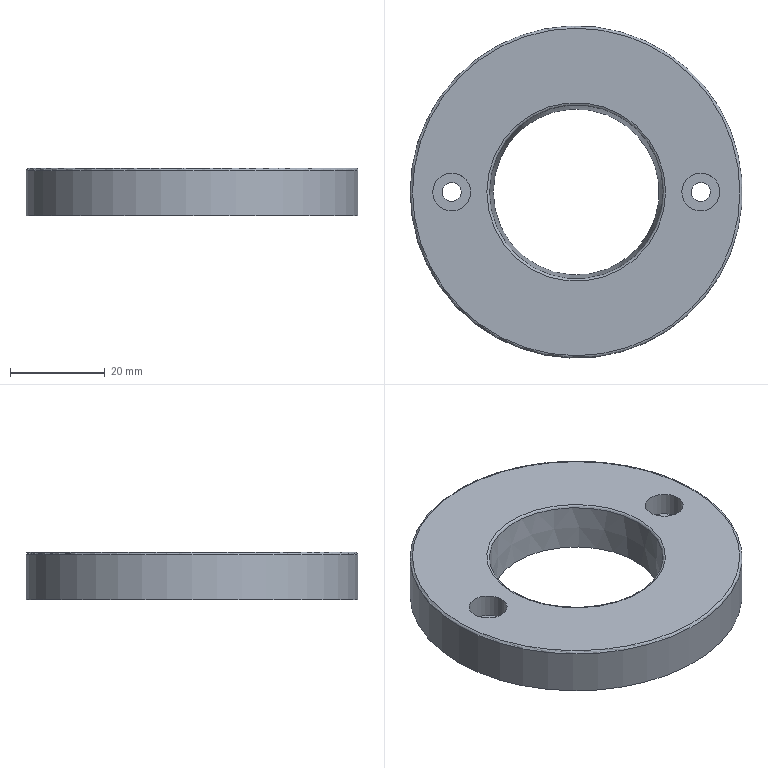Part | STEP file | DISCO_BASE_ALIMENTADOR_ARRUELA | 1 solid | 12 faces | box 70 x 70 x 10 mm | volume 27729 mm3 | cylinder 5 | plane 4 | torus 2 | cone 1 | commonest cylinder face diameters 4 x2 8 x2 70 x1
STEP:
#1=CARTESIAN_POINT('',(0.,0.,0.));
#2=DIRECTION('',(0.,0.,1.));
#3=DIRECTION('',(1.,0.,0.));
#4=AXIS2_PLACEMENT_3D('',#1,#2,#3);
#5=CARTESIAN_POINT('',(-29.76,1.918,5.));
#6=VERTEX_POINT('',#5);
#7=CARTESIAN_POINT('',(-26.25,0.,5.));
#8=DIRECTION('',(0.,0.,-1.));
#9=DIRECTION('',(1.,0.,0.));
#10=AXIS2_PLACEMENT_3D('',#7,#8,#9);
#11=CIRCLE('',#10,4.);
#12=CARTESIAN_POINT('',(-24.25,0.,5.));
#13=DIRECTION('',(0.,0.,-1.));
#14=DIRECTION('',(-1.,0.,0.));
#15=AXIS2_PLACEMENT_3D('',#12,#13,#14);
#16=PLANE('',#15);
#17=CARTESIAN_POINT('',(2.,0.));
#18=DIRECTION('',(-1.,0.));
#19=AXIS2_PLACEMENT_2D('',#17,#18);
#20=CIRCLE('',#19,4.);
#21=(GEOMETRIC_REPRESENTATION_CONTEXT(2)PARAMETRIC_REPRESENTATION_CONTEXT()REPRESENTATION_CONTEXT('',''));
#22=DEFINITIONAL_REPRESENTATION('',(#20),#21);
#23=PCURVE('',#16,#22);
#24=CARTESIAN_POINT('',(-26.25,0.,9.9));
#25=DIRECTION('',(0.,0.,-1.));
#26=DIRECTION('',(0.8776,-0.4794,0.));
#27=AXIS2_PLACEMENT_3D('',#24,#25,#26);
#28=CYLINDRICAL_SURFACE('',#27,4.);
#29=CARTESIAN_POINT('',(-0.5,4.9));
#30=DIRECTION('',(1.,0.));
#31=VECTOR('',#30,1.);
#32=LINE('',#29,#31);
#33=(GEOMETRIC_REPRESENTATION_CONTEXT(2)PARAMETRIC_REPRESENTATION_CONTEXT()REPRESENTATION_CONTEXT('',''));
#34=DEFINITIONAL_REPRESENTATION('',(#32),#33);
#35=PCURVE('',#28,#34);
#36=SURFACE_CURVE('',#11,(#23,#35),.PCURVE_S1.);
#37=EDGE_CURVE('',#6,#6,#36,.T.);
#38=ORIENTED_EDGE('',*,*,#37,.F.);
#39=EDGE_LOOP('',(#38));
#40=FACE_BOUND('',#39,.T.);
#41=CARTESIAN_POINT('',(-24.495,-0.9589,5.));
#42=VERTEX_POINT('',#41);
#43=CARTESIAN_POINT('',(-26.25,0.,5.));
#44=DIRECTION('',(0.,0.,-1.));
#45=DIRECTION('',(1.,0.,0.));
#46=AXIS2_PLACEMENT_3D('',#43,#44,#45);
#47=CIRCLE('',#46,2.);
#48=CARTESIAN_POINT('',(2.,0.));
#49=DIRECTION('',(-1.,0.));
#50=AXIS2_PLACEMENT_2D('',#48,#49);
#51=CIRCLE('',#50,2.);
#52=(GEOMETRIC_REPRESENTATION_CONTEXT(2)PARAMETRIC_REPRESENTATION_CONTEXT()REPRESENTATION_CONTEXT('',''));
#53=DEFINITIONAL_REPRESENTATION('',(#51),#52);
#54=PCURVE('',#16,#53);
#55=CARTESIAN_POINT('',(-26.25,0.,9.9));
#56=DIRECTION('',(0.,0.,-1.));
#57=DIRECTION('',(0.8776,-0.4794,0.));
#58=AXIS2_PLACEMENT_3D('',#55,#56,#57);
#59=CYLINDRICAL_SURFACE('',#58,2.);
#60=CARTESIAN_POINT('',(-0.5,4.9));
#61=DIRECTION('',(1.,0.));
#62=VECTOR('',#61,1.);
#63=LINE('',#60,#62);
#64=(GEOMETRIC_REPRESENTATION_CONTEXT(2)PARAMETRIC_REPRESENTATION_CONTEXT()REPRESENTATION_CONTEXT('',''));
#65=DEFINITIONAL_REPRESENTATION('',(#63),#64);
#66=PCURVE('',#59,#65);
#67=SURFACE_CURVE('',#47,(#54,#66),.PCURVE_S1.);
#68=EDGE_CURVE('',#42,#42,#67,.T.);
#69=ORIENTED_EDGE('',*,*,#68,.T.);
#70=EDGE_LOOP('',(#69));
#71=FACE_BOUND('',#70,.T.);
#72=ADVANCED_FACE('',(#40,#71),#16,.F.);
#73=CARTESIAN_POINT('',(-24.495,-0.9589,0.));
#74=VERTEX_POINT('',#73);
#75=CARTESIAN_POINT('',(-26.25,0.,0.));
#76=DIRECTION('',(0.,0.,-1.));
#77=DIRECTION('',(1.,0.,0.));
#78=AXIS2_PLACEMENT_3D('',#75,#76,#77);
#79=CIRCLE('',#78,2.);
#80=CARTESIAN_POINT('',(-0.5,9.9));
#81=DIRECTION('',(1.,0.));
#82=VECTOR('',#81,1.);
#83=LINE('',#80,#82);
#84=(GEOMETRIC_REPRESENTATION_CONTEXT(2)PARAMETRIC_REPRESENTATION_CONTEXT()REPRESENTATION_CONTEXT('',''));
#85=DEFINITIONAL_REPRESENTATION('',(#83),#84);
#86=PCURVE('',#59,#85);
#87=CARTESIAN_POINT('',(0.,0.,0.));
#88=DIRECTION('',(0.,0.,1.));
#89=DIRECTION('',(1.,0.,0.));
#90=AXIS2_PLACEMENT_3D('',#87,#88,#89);
#91=PLANE('',#90);
#92=CARTESIAN_POINT('',(-24.25,0.));
#93=CARTESIAN_POINT('',(-24.25,-3.464));
#94=CARTESIAN_POINT('',(-27.25,-1.732));
#95=CARTESIAN_POINT('',(-30.25,0.));
#96=CARTESIAN_POINT('',(-27.25,1.732));
#97=CARTESIAN_POINT('',(-24.25,3.464));
#98=CARTESIAN_POINT('',(-24.25,0.));
#99=(BOUNDED_CURVE()B_SPLINE_CURVE(2,(#92,#93,#94,#95,#96,#97,#98),.UNSPECIFIED.,.T.,.F.)B_SPLINE_CURVE_WITH_KNOTS((1,2,2,2,2,1),(-2.094,0.,2.094,4.189,6.283,8.378),.UNSPECIFIED.)CURVE()GEOMETRIC_REPRESENTATION_ITEM()RATIONAL_B_SPLINE_CURVE((1.,0.5,1.,0.5,1.,0.5,1.))REPRESENTATION_ITEM(''));
#100=(GEOMETRIC_REPRESENTATION_CONTEXT(2)PARAMETRIC_REPRESENTATION_CONTEXT()REPRESENTATION_CONTEXT('',''));
#101=DEFINITIONAL_REPRESENTATION('',(#99),#100);
#102=PCURVE('',#91,#101);
#103=SURFACE_CURVE('',#79,(#86,#102),.PCURVE_S1.);
#104=EDGE_CURVE('',#74,#74,#103,.T.);
#105=ORIENTED_EDGE('',*,*,#104,.F.);
#106=CARTESIAN_POINT('',(-24.495,-0.9589,5.));
#107=CARTESIAN_POINT('',(-24.495,-0.9589,0.));
#108=B_SPLINE_CURVE_WITH_KNOTS('',1,(#106,#107),.UNSPECIFIED.,.F.,.F.,(2,2),(4.9,9.9),.PIECEWISE_BEZIER_KNOTS.);
#109=CARTESIAN_POINT('',(0.,0.));
#110=DIRECTION('',(0.,1.));
#111=VECTOR('',#110,1.);
#112=LINE('',#109,#111);
#113=(GEOMETRIC_REPRESENTATION_CONTEXT(2)PARAMETRIC_REPRESENTATION_CONTEXT()REPRESENTATION_CONTEXT('',''));
#114=DEFINITIONAL_REPRESENTATION('',(#112),#113);
#115=PCURVE('',#59,#114);
#116=CARTESIAN_POINT('',(6.283,0.));
#117=DIRECTION('',(0.,1.));
#118=VECTOR('',#117,1.);
#119=LINE('',#116,#118);
#120=(GEOMETRIC_REPRESENTATION_CONTEXT(2)PARAMETRIC_REPRESENTATION_CONTEXT()REPRESENTATION_CONTEXT('',''));
#121=DEFINITIONAL_REPRESENTATION('',(#119),#120);
#122=PCURVE('',#59,#121);
#123=SEAM_CURVE('',#108,(#115,#122),.PCURVE_S1.);
#124=EDGE_CURVE('',#42,#74,#123,.T.);
#125=ORIENTED_EDGE('',*,*,#124,.F.);
#126=ORIENTED_EDGE('',*,*,#68,.T.);
#127=ORIENTED_EDGE('',*,*,#124,.T.);
#128=EDGE_LOOP('',(#105,#125,#126,#127));
#129=FACE_BOUND('',#128,.F.);
#130=ADVANCED_FACE('',(#129),#59,.F.);
#131=CARTESIAN_POINT('',(-29.76,1.918,10.));
#132=VERTEX_POINT('',#131);
#133=CARTESIAN_POINT('',(-26.25,0.,10.));
#134=DIRECTION('',(0.,0.,-1.));
#135=DIRECTION('',(1.,0.,0.));
#136=AXIS2_PLACEMENT_3D('',#133,#134,#135);
#137=CIRCLE('',#136,4.);
#138=CARTESIAN_POINT('',(-0.5,-0.1));
#139=DIRECTION('',(1.,0.));
#140=VECTOR('',#139,1.);
#141=LINE('',#138,#140);
#142=(GEOMETRIC_REPRESENTATION_CONTEXT(2)PARAMETRIC_REPRESENTATION_CONTEXT()REPRESENTATION_CONTEXT('',''));
#143=DEFINITIONAL_REPRESENTATION('',(#141),#142);
#144=PCURVE('',#28,#143);
#145=CARTESIAN_POINT('',(0.,0.,10.));
#146=DIRECTION('',(0.,0.,1.));
#147=DIRECTION('',(1.,0.,0.));
#148=AXIS2_PLACEMENT_3D('',#145,#146,#147);
#149=PLANE('',#148);
#150=CARTESIAN_POINT('',(-22.25,0.));
#151=CARTESIAN_POINT('',(-22.25,-6.928));
#152=CARTESIAN_POINT('',(-28.25,-3.464));
#153=CARTESIAN_POINT('',(-34.25,0.));
#154=CARTESIAN_POINT('',(-28.25,3.464));
#155=CARTESIAN_POINT('',(-22.25,6.928));
#156=CARTESIAN_POINT('',(-22.25,0.));
#157=(BOUNDED_CURVE()B_SPLINE_CURVE(2,(#150,#151,#152,#153,#154,#155,#156),.UNSPECIFIED.,.T.,.F.)B_SPLINE_CURVE_WITH_KNOTS((1,2,2,2,2,1),(-2.094,0.,2.094,4.189,6.283,8.378),.UNSPECIFIED.)CURVE()GEOMETRIC_REPRESENTATION_ITEM()RATIONAL_B_SPLINE_CURVE((1.,0.5,1.,0.5,1.,0.5,1.))REPRESENTATION_ITEM(''));
#158=(GEOMETRIC_REPRESENTATION_CONTEXT(2)PARAMETRIC_REPRESENTATION_CONTEXT()REPRESENTATION_CONTEXT('',''));
#159=DEFINITIONAL_REPRESENTATION('',(#157),#158);
#160=PCURVE('',#149,#159);
#161=SURFACE_CURVE('',#137,(#144,#160),.PCURVE_S1.);
#162=EDGE_CURVE('',#132,#132,#161,.T.);
#163=ORIENTED_EDGE('',*,*,#162,.T.);
#164=CARTESIAN_POINT('',(-29.76,1.918,10.));
#165=CARTESIAN_POINT('',(-29.76,1.918,5.));
#166=B_SPLINE_CURVE_WITH_KNOTS('',1,(#164,#165),.UNSPECIFIED.,.F.,.F.,(2,2),(-0.1,4.9),.PIECEWISE_BEZIER_KNOTS.);
#167=CARTESIAN_POINT('',(9.425,0.));
#168=DIRECTION('',(0.,1.));
#169=VECTOR('',#168,1.);
#170=LINE('',#167,#169);
#171=(GEOMETRIC_REPRESENTATION_CONTEXT(2)PARAMETRIC_REPRESENTATION_CONTEXT()REPRESENTATION_CONTEXT('',''));
#172=DEFINITIONAL_REPRESENTATION('',(#170),#171);
#173=PCURVE('',#28,#172);
#174=CARTESIAN_POINT('',(3.142,0.));
#175=DIRECTION('',(0.,1.));
#176=VECTOR('',#175,1.);
#177=LINE('',#174,#176);
#178=(GEOMETRIC_REPRESENTATION_CONTEXT(2)PARAMETRIC_REPRESENTATION_CONTEXT()REPRESENTATION_CONTEXT('',''));
#179=DEFINITIONAL_REPRESENTATION('',(#177),#178);
#180=PCURVE('',#28,#179);
#181=SEAM_CURVE('',#166,(#173,#180),.PCURVE_S1.);
#182=EDGE_CURVE('',#132,#6,#181,.T.);
#183=ORIENTED_EDGE('',*,*,#182,.T.);
#184=ORIENTED_EDGE('',*,*,#37,.F.);
#185=ORIENTED_EDGE('',*,*,#182,.F.);
#186=EDGE_LOOP('',(#163,#183,#184,#185));
#187=FACE_BOUND('',#186,.F.);
#188=ADVANCED_FACE('',(#187),#28,.F.);
#189=CARTESIAN_POINT('',(-35.,0.,0.));
#190=VERTEX_POINT('',#189);
#191=CARTESIAN_POINT('',(0.,0.,0.));
#192=DIRECTION('',(0.,0.,1.));
#193=DIRECTION('',(1.,0.,0.));
#194=AXIS2_PLACEMENT_3D('',#191,#192,#193);
#195=CIRCLE('',#194,35.);
#196=CARTESIAN_POINT('',(0.,0.));
#197=DIRECTION('',(1.,0.));
#198=AXIS2_PLACEMENT_2D('',#196,#197);
#199=CIRCLE('',#198,35.);
#200=(GEOMETRIC_REPRESENTATION_CONTEXT(2)PARAMETRIC_REPRESENTATION_CONTEXT()REPRESENTATION_CONTEXT('',''));
#201=DEFINITIONAL_REPRESENTATION('',(#199),#200);
#202=PCURVE('',#91,#201);
#203=CARTESIAN_POINT('',(0.,0.,5.));
#204=DIRECTION('',(0.,0.,1.));
#205=DIRECTION('',(1.,0.,0.));
#206=AXIS2_PLACEMENT_3D('',#203,#204,#205);
#207=CYLINDRICAL_SURFACE('',#206,35.);
#208=CARTESIAN_POINT('',(0.,-5.));
#209=DIRECTION('',(1.,0.));
#210=VECTOR('',#209,1.);
#211=LINE('',#208,#210);
#212=(GEOMETRIC_REPRESENTATION_CONTEXT(2)PARAMETRIC_REPRESENTATION_CONTEXT()REPRESENTATION_CONTEXT('',''));
#213=DEFINITIONAL_REPRESENTATION('',(#211),#212);
#214=PCURVE('',#207,#213);
#215=SURFACE_CURVE('',#195,(#202,#214),.PCURVE_S1.);
#216=EDGE_CURVE('',#190,#190,#215,.T.);
#217=ORIENTED_EDGE('',*,*,#216,.F.);
#218=EDGE_LOOP('',(#217));
#219=FACE_BOUND('',#218,.T.);
#220=CARTESIAN_POINT('',(24.495,0.9589,0.));
#221=VERTEX_POINT('',#220);
#222=CARTESIAN_POINT('',(26.25,0.,0.));
#223=DIRECTION('',(0.,0.,1.));
#224=DIRECTION('',(1.,0.,0.));
#225=AXIS2_PLACEMENT_3D('',#222,#223,#224);
#226=CIRCLE('',#225,2.);
#227=CARTESIAN_POINT('',(26.25,0.));
#228=DIRECTION('',(1.,0.));
#229=AXIS2_PLACEMENT_2D('',#227,#228);
#230=CIRCLE('',#229,2.);
#231=(GEOMETRIC_REPRESENTATION_CONTEXT(2)PARAMETRIC_REPRESENTATION_CONTEXT()REPRESENTATION_CONTEXT('',''));
#232=DEFINITIONAL_REPRESENTATION('',(#230),#231);
#233=PCURVE('',#91,#232);
#234=CARTESIAN_POINT('',(26.25,0.,9.9));
#235=DIRECTION('',(0.,0.,-1.));
#236=DIRECTION('',(-0.8776,0.4794,0.));
#237=AXIS2_PLACEMENT_3D('',#234,#235,#236);
#238=CYLINDRICAL_SURFACE('',#237,2.);
#239=CARTESIAN_POINT('',(8.925,9.9));
#240=DIRECTION('',(-1.,0.));
#241=VECTOR('',#240,1.);
#242=LINE('',#239,#241);
#243=(GEOMETRIC_REPRESENTATION_CONTEXT(2)PARAMETRIC_REPRESENTATION_CONTEXT()REPRESENTATION_CONTEXT('',''));
#244=DEFINITIONAL_REPRESENTATION('',(#242),#243);
#245=PCURVE('',#238,#244);
#246=SURFACE_CURVE('',#226,(#233,#245),.PCURVE_S1.);
#247=EDGE_CURVE('',#221,#221,#246,.T.);
#248=ORIENTED_EDGE('',*,*,#247,.T.);
#249=EDGE_LOOP('',(#248));
#250=FACE_BOUND('',#249,.T.);
#251=ORIENTED_EDGE('',*,*,#104,.F.);
#252=EDGE_LOOP('',(#251));
#253=FACE_BOUND('',#252,.T.);
#254=CARTESIAN_POINT('',(-17.5,0.,0.));
#255=VERTEX_POINT('',#254);
#256=CARTESIAN_POINT('',(0.,0.,0.));
#257=DIRECTION('',(0.,0.,1.));
#258=DIRECTION('',(1.,0.,0.));
#259=AXIS2_PLACEMENT_3D('',#256,#257,#258);
#260=CIRCLE('',#259,17.5);
#261=CARTESIAN_POINT('',(0.,0.));
#262=DIRECTION('',(1.,0.));
#263=AXIS2_PLACEMENT_2D('',#261,#262);
#264=CIRCLE('',#263,17.5);
#265=(GEOMETRIC_REPRESENTATION_CONTEXT(2)PARAMETRIC_REPRESENTATION_CONTEXT()REPRESENTATION_CONTEXT('',''));
#266=DEFINITIONAL_REPRESENTATION('',(#264),#265);
#267=PCURVE('',#91,#266);
#268=CARTESIAN_POINT('',(0.,0.,0.));
#269=DIRECTION('',(0.,0.,1.));
#270=DIRECTION('',(-1.,0.,0.));
#271=AXIS2_PLACEMENT_3D('',#268,#269,#270);
#272=CONICAL_SURFACE('',#271,17.5,0.08727);
#273=CARTESIAN_POINT('',(-3.142,0.));
#274=DIRECTION('',(1.,0.));
#275=VECTOR('',#274,1.);
#276=LINE('',#273,#275);
#277=(GEOMETRIC_REPRESENTATION_CONTEXT(2)PARAMETRIC_REPRESENTATION_CONTEXT()REPRESENTATION_CONTEXT('',''));
#278=DEFINITIONAL_REPRESENTATION('',(#276),#277);
#279=PCURVE('',#272,#278);
#280=SURFACE_CURVE('',#260,(#267,#279),.PCURVE_S1.);
#281=EDGE_CURVE('',#255,#255,#280,.T.);
#282=ORIENTED_EDGE('',*,*,#281,.T.);
#283=EDGE_LOOP('',(#282));
#284=FACE_BOUND('',#283,.T.);
#285=ADVANCED_FACE('',(#219,#250,#253,#284),#91,.F.);
#286=CARTESIAN_POINT('',(22.74,1.918,5.));
#287=VERTEX_POINT('',#286);
#288=CARTESIAN_POINT('',(26.25,0.,5.));
#289=DIRECTION('',(0.,0.,-1.));
#290=DIRECTION('',(1.,0.,0.));
#291=AXIS2_PLACEMENT_3D('',#288,#289,#290);
#292=CIRCLE('',#291,4.);
#293=CARTESIAN_POINT('',(-24.25,0.,5.));
#294=DIRECTION('',(0.,0.,-1.));
#295=DIRECTION('',(-1.,0.,0.));
#296=AXIS2_PLACEMENT_3D('',#293,#294,#295);
#297=PLANE('',#296);
#298=CARTESIAN_POINT('',(-50.5,0.));
#299=DIRECTION('',(-1.,0.));
#300=AXIS2_PLACEMENT_2D('',#298,#299);
#301=CIRCLE('',#300,4.);
#302=(GEOMETRIC_REPRESENTATION_CONTEXT(2)PARAMETRIC_REPRESENTATION_CONTEXT()REPRESENTATION_CONTEXT('',''));
#303=DEFINITIONAL_REPRESENTATION('',(#301),#302);
#304=PCURVE('',#297,#303);
#305=CARTESIAN_POINT('',(26.25,0.,9.9));
#306=DIRECTION('',(0.,0.,-1.));
#307=DIRECTION('',(-0.8776,0.4794,0.));
#308=AXIS2_PLACEMENT_3D('',#305,#306,#307);
#309=CYLINDRICAL_SURFACE('',#308,4.);
#310=CARTESIAN_POINT('',(-3.642,4.9));
#311=DIRECTION('',(1.,0.));
#312=VECTOR('',#311,1.);
#313=LINE('',#310,#312);
#314=(GEOMETRIC_REPRESENTATION_CONTEXT(2)PARAMETRIC_REPRESENTATION_CONTEXT()REPRESENTATION_CONTEXT('',''));
#315=DEFINITIONAL_REPRESENTATION('',(#313),#314);
#316=PCURVE('',#309,#315);
#317=SURFACE_CURVE('',#292,(#304,#316),.PCURVE_S1.);
#318=EDGE_CURVE('',#287,#287,#317,.T.);
#319=ORIENTED_EDGE('',*,*,#318,.F.);
#320=EDGE_LOOP('',(#319));
#321=FACE_BOUND('',#320,.T.);
#322=CARTESIAN_POINT('',(24.495,0.9589,5.));
#323=VERTEX_POINT('',#322);
#324=CARTESIAN_POINT('',(26.25,0.,5.));
#325=DIRECTION('',(0.,0.,-1.));
#326=DIRECTION('',(1.,0.,0.));
#327=AXIS2_PLACEMENT_3D('',#324,#325,#326);
#328=CIRCLE('',#327,2.);
#329=CARTESIAN_POINT('',(-50.5,0.));
#330=DIRECTION('',(-1.,0.));
#331=AXIS2_PLACEMENT_2D('',#329,#330);
#332=CIRCLE('',#331,2.);
#333=(GEOMETRIC_REPRESENTATION_CONTEXT(2)PARAMETRIC_REPRESENTATION_CONTEXT()REPRESENTATION_CONTEXT('',''));
#334=DEFINITIONAL_REPRESENTATION('',(#332),#333);
#335=PCURVE('',#297,#334);
#336=CARTESIAN_POINT('',(-3.642,4.9));
#337=DIRECTION('',(1.,0.));
#338=VECTOR('',#337,1.);
#339=LINE('',#336,#338);
#340=(GEOMETRIC_REPRESENTATION_CONTEXT(2)PARAMETRIC_REPRESENTATION_CONTEXT()REPRESENTATION_CONTEXT('',''));
#341=DEFINITIONAL_REPRESENTATION('',(#339),#340);
#342=PCURVE('',#238,#341);
#343=SURFACE_CURVE('',#328,(#335,#342),.PCURVE_S1.);
#344=EDGE_CURVE('',#323,#323,#343,.T.);
#345=ORIENTED_EDGE('',*,*,#344,.T.);
#346=EDGE_LOOP('',(#345));
#347=FACE_BOUND('',#346,.T.);
#348=ADVANCED_FACE('',(#321,#347),#297,.F.);
#349=CARTESIAN_POINT('',(22.74,1.918,10.));
#350=VERTEX_POINT('',#349);
#351=CARTESIAN_POINT('',(26.25,0.,10.));
#352=DIRECTION('',(0.,0.,-1.));
#353=DIRECTION('',(1.,0.,0.));
#354=AXIS2_PLACEMENT_3D('',#351,#352,#353);
#355=CIRCLE('',#354,4.);
#356=CARTESIAN_POINT('',(-3.642,-0.1));
#357=DIRECTION('',(1.,0.));
#358=VECTOR('',#357,1.);
#359=LINE('',#356,#358);
#360=(GEOMETRIC_REPRESENTATION_CONTEXT(2)PARAMETRIC_REPRESENTATION_CONTEXT()REPRESENTATION_CONTEXT('',''));
#361=DEFINITIONAL_REPRESENTATION('',(#359),#360);
#362=PCURVE('',#309,#361);
#363=CARTESIAN_POINT('',(30.25,0.));
#364=CARTESIAN_POINT('',(30.25,-6.928));
#365=CARTESIAN_POINT('',(24.25,-3.464));
#366=CARTESIAN_POINT('',(18.25,0.));
#367=CARTESIAN_POINT('',(24.25,3.464));
#368=CARTESIAN_POINT('',(30.25,6.928));
#369=CARTESIAN_POINT('',(30.25,0.));
#370=(BOUNDED_CURVE()B_SPLINE_CURVE(2,(#363,#364,#365,#366,#367,#368,#369),.UNSPECIFIED.,.T.,.F.)B_SPLINE_CURVE_WITH_KNOTS((1,2,2,2,2,1),(-2.094,0.,2.094,4.189,6.283,8.378),.UNSPECIFIED.)CURVE()GEOMETRIC_REPRESENTATION_ITEM()RATIONAL_B_SPLINE_CURVE((1.,0.5,1.,0.5,1.,0.5,1.))REPRESENTATION_ITEM(''));
#371=(GEOMETRIC_REPRESENTATION_CONTEXT(2)PARAMETRIC_REPRESENTATION_CONTEXT()REPRESENTATION_CONTEXT('',''));
#372=DEFINITIONAL_REPRESENTATION('',(#370),#371);
#373=PCURVE('',#149,#372);
#374=SURFACE_CURVE('',#355,(#362,#373),.PCURVE_S1.);
#375=EDGE_CURVE('',#350,#350,#374,.T.);
#376=ORIENTED_EDGE('',*,*,#375,.T.);
#377=CARTESIAN_POINT('',(22.74,1.918,10.));
#378=CARTESIAN_POINT('',(22.74,1.918,5.));
#379=B_SPLINE_CURVE_WITH_KNOTS('',1,(#377,#378),.UNSPECIFIED.,.F.,.F.,(2,2),(-0.1,4.9),.PIECEWISE_BEZIER_KNOTS.);
#380=CARTESIAN_POINT('',(6.283,0.));
#381=DIRECTION('',(0.,1.));
#382=VECTOR('',#381,1.);
#383=LINE('',#380,#382);
#384=(GEOMETRIC_REPRESENTATION_CONTEXT(2)PARAMETRIC_REPRESENTATION_CONTEXT()REPRESENTATION_CONTEXT('',''));
#385=DEFINITIONAL_REPRESENTATION('',(#383),#384);
#386=PCURVE('',#309,#385);
#387=CARTESIAN_POINT('',(0.,0.));
#388=DIRECTION('',(0.,1.));
#389=VECTOR('',#388,1.);
#390=LINE('',#387,#389);
#391=(GEOMETRIC_REPRESENTATION_CONTEXT(2)PARAMETRIC_REPRESENTATION_CONTEXT()REPRESENTATION_CONTEXT('',''));
#392=DEFINITIONAL_REPRESENTATION('',(#390),#391);
#393=PCURVE('',#309,#392);
#394=SEAM_CURVE('',#379,(#386,#393),.PCURVE_S1.);
#395=EDGE_CURVE('',#350,#287,#394,.T.);
#396=ORIENTED_EDGE('',*,*,#395,.T.);
#397=ORIENTED_EDGE('',*,*,#318,.F.);
#398=ORIENTED_EDGE('',*,*,#395,.F.);
#399=EDGE_LOOP('',(#376,#396,#397,#398));
#400=FACE_BOUND('',#399,.F.);
#401=ADVANCED_FACE('',(#400),#309,.F.);
#402=ORIENTED_EDGE('',*,*,#247,.T.);
#403=CARTESIAN_POINT('',(24.495,0.9589,5.));
#404=CARTESIAN_POINT('',(24.495,0.9589,0.));
#405=B_SPLINE_CURVE_WITH_KNOTS('',1,(#403,#404),.UNSPECIFIED.,.F.,.F.,(2,2),(4.9,9.9),.PIECEWISE_BEZIER_KNOTS.);
#406=CARTESIAN_POINT('',(0.,0.));
#407=DIRECTION('',(0.,1.));
#408=VECTOR('',#407,1.);
#409=LINE('',#406,#408);
#410=(GEOMETRIC_REPRESENTATION_CONTEXT(2)PARAMETRIC_REPRESENTATION_CONTEXT()REPRESENTATION_CONTEXT('',''));
#411=DEFINITIONAL_REPRESENTATION('',(#409),#410);
#412=PCURVE('',#238,#411);
#413=CARTESIAN_POINT('',(6.283,0.));
#414=DIRECTION('',(0.,1.));
#415=VECTOR('',#414,1.);
#416=LINE('',#413,#415);
#417=(GEOMETRIC_REPRESENTATION_CONTEXT(2)PARAMETRIC_REPRESENTATION_CONTEXT()REPRESENTATION_CONTEXT('',''));
#418=DEFINITIONAL_REPRESENTATION('',(#416),#417);
#419=PCURVE('',#238,#418);
#420=SEAM_CURVE('',#405,(#412,#419),.PCURVE_S1.);
#421=EDGE_CURVE('',#323,#221,#420,.T.);
#422=ORIENTED_EDGE('',*,*,#421,.F.);
#423=ORIENTED_EDGE('',*,*,#344,.T.);
#424=ORIENTED_EDGE('',*,*,#421,.T.);
#425=EDGE_LOOP('',(#402,#422,#423,#424));
#426=FACE_BOUND('',#425,.F.);
#427=ADVANCED_FACE('',(#426),#238,.F.);
#428=CARTESIAN_POINT('',(-35.,0.,9.5));
#429=VERTEX_POINT('',#428);
#430=CARTESIAN_POINT('',(0.,0.,9.5));
#431=DIRECTION('',(0.,0.,1.));
#432=DIRECTION('',(1.,0.,0.));
#433=AXIS2_PLACEMENT_3D('',#430,#431,#432);
#434=CIRCLE('',#433,35.);
#435=CARTESIAN_POINT('',(0.,4.5));
#436=DIRECTION('',(1.,0.));
#437=VECTOR('',#436,1.);
#438=LINE('',#435,#437);
#439=(GEOMETRIC_REPRESENTATION_CONTEXT(2)PARAMETRIC_REPRESENTATION_CONTEXT()REPRESENTATION_CONTEXT('',''));
#440=DEFINITIONAL_REPRESENTATION('',(#438),#439);
#441=PCURVE('',#207,#440);
#442=CARTESIAN_POINT('',(0.,0.,9.5));
#443=DIRECTION('',(0.,0.,1.));
#444=DIRECTION('',(1.,0.,0.));
#445=AXIS2_PLACEMENT_3D('',#442,#443,#444);
#446=TOROIDAL_SURFACE('',#445,34.5,0.5);
#447=CARTESIAN_POINT('',(0.,6.283));
#448=DIRECTION('',(1.,0.));
#449=VECTOR('',#448,1.);
#450=LINE('',#447,#449);
#451=(GEOMETRIC_REPRESENTATION_CONTEXT(2)PARAMETRIC_REPRESENTATION_CONTEXT()REPRESENTATION_CONTEXT('',''));
#452=DEFINITIONAL_REPRESENTATION('',(#450),#451);
#453=PCURVE('',#446,#452);
#454=SURFACE_CURVE('',#434,(#441,#453),.PCURVE_S1.);
#455=EDGE_CURVE('',#429,#429,#454,.T.);
#456=ORIENTED_EDGE('',*,*,#455,.F.);
#457=CARTESIAN_POINT('',(-35.,0.,0.));
#458=CARTESIAN_POINT('',(-35.,0.,9.5));
#459=B_SPLINE_CURVE_WITH_KNOTS('',1,(#457,#458),.UNSPECIFIED.,.F.,.F.,(2,2),(-5.,4.5),.PIECEWISE_BEZIER_KNOTS.);
#460=CARTESIAN_POINT('',(3.142,0.));
#461=DIRECTION('',(0.,1.));
#462=VECTOR('',#461,1.);
#463=LINE('',#460,#462);
#464=(GEOMETRIC_REPRESENTATION_CONTEXT(2)PARAMETRIC_REPRESENTATION_CONTEXT()REPRESENTATION_CONTEXT('',''));
#465=DEFINITIONAL_REPRESENTATION('',(#463),#464);
#466=PCURVE('',#207,#465);
#467=CARTESIAN_POINT('',(9.425,0.));
#468=DIRECTION('',(0.,1.));
#469=VECTOR('',#468,1.);
#470=LINE('',#467,#469);
#471=(GEOMETRIC_REPRESENTATION_CONTEXT(2)PARAMETRIC_REPRESENTATION_CONTEXT()REPRESENTATION_CONTEXT('',''));
#472=DEFINITIONAL_REPRESENTATION('',(#470),#471);
#473=PCURVE('',#207,#472);
#474=SEAM_CURVE('',#459,(#466,#473),.PCURVE_S1.);
#475=EDGE_CURVE('',#190,#429,#474,.T.);
#476=ORIENTED_EDGE('',*,*,#475,.F.);
#477=ORIENTED_EDGE('',*,*,#216,.T.);
#478=ORIENTED_EDGE('',*,*,#475,.T.);
#479=EDGE_LOOP('',(#456,#476,#477,#478));
#480=FACE_BOUND('',#479,.T.);
#481=ADVANCED_FACE('',(#480),#207,.T.);
#482=CARTESIAN_POINT('',(-34.5,-0.000000018,10.));
#483=VERTEX_POINT('',#482);
#484=CARTESIAN_POINT('',(0.,0.,10.));
#485=DIRECTION('',(0.,0.,1.));
#486=DIRECTION('',(1.,0.,0.));
#487=AXIS2_PLACEMENT_3D('',#484,#485,#486);
#488=CIRCLE('',#487,34.5);
#489=CARTESIAN_POINT('',(0.,7.854));
#490=DIRECTION('',(1.,0.));
#491=VECTOR('',#490,1.);
#492=LINE('',#489,#491);
#493=(GEOMETRIC_REPRESENTATION_CONTEXT(2)PARAMETRIC_REPRESENTATION_CONTEXT()REPRESENTATION_CONTEXT('',''));
#494=DEFINITIONAL_REPRESENTATION('',(#492),#493);
#495=PCURVE('',#446,#494);
#496=CARTESIAN_POINT('',(0.,0.));
#497=DIRECTION('',(1.,0.));
#498=AXIS2_PLACEMENT_2D('',#496,#497);
#499=CIRCLE('',#498,34.5);
#500=(GEOMETRIC_REPRESENTATION_CONTEXT(2)PARAMETRIC_REPRESENTATION_CONTEXT()REPRESENTATION_CONTEXT('',''));
#501=DEFINITIONAL_REPRESENTATION('',(#499),#500);
#502=PCURVE('',#149,#501);
#503=SURFACE_CURVE('',#488,(#495,#502),.PCURVE_S1.);
#504=EDGE_CURVE('',#483,#483,#503,.T.);
#505=ORIENTED_EDGE('',*,*,#504,.F.);
#506=CARTESIAN_POINT('',(-35.,-0.000000019,9.5));
#507=CARTESIAN_POINT('',(-35.,-0.000000019,9.634));
#508=CARTESIAN_POINT('',(-34.957,-0.000000019,9.764));
#509=CARTESIAN_POINT('',(-34.876,-0.000000019,9.876));
#510=CARTESIAN_POINT('',(-34.764,-0.000000019,9.957));
#511=CARTESIAN_POINT('',(-34.634,-0.000000018,10.));
#512=CARTESIAN_POINT('',(-34.5,-0.000000018,10.));
#513=(BOUNDED_CURVE()B_SPLINE_CURVE(6,(#506,#507,#508,#509,#510,#511,#512),.UNSPECIFIED.,.F.,.F.)B_SPLINE_CURVE_WITH_KNOTS((7,7),(0.,1.571),.PIECEWISE_BEZIER_KNOTS.)CURVE()GEOMETRIC_REPRESENTATION_ITEM()RATIONAL_B_SPLINE_CURVE((1.031,1.01,0.9979,0.994,0.9979,1.01,1.031))REPRESENTATION_ITEM(''));
#514=CARTESIAN_POINT('',(3.142,6.283));
#515=DIRECTION('',(0.,1.));
#516=VECTOR('',#515,1.);
#517=LINE('',#514,#516);
#518=(GEOMETRIC_REPRESENTATION_CONTEXT(2)PARAMETRIC_REPRESENTATION_CONTEXT()REPRESENTATION_CONTEXT('',''));
#519=DEFINITIONAL_REPRESENTATION('',(#517),#518);
#520=PCURVE('',#446,#519);
#521=CARTESIAN_POINT('',(9.425,6.283));
#522=DIRECTION('',(0.,1.));
#523=VECTOR('',#522,1.);
#524=LINE('',#521,#523);
#525=(GEOMETRIC_REPRESENTATION_CONTEXT(2)PARAMETRIC_REPRESENTATION_CONTEXT()REPRESENTATION_CONTEXT('',''));
#526=DEFINITIONAL_REPRESENTATION('',(#524),#525);
#527=PCURVE('',#446,#526);
#528=SEAM_CURVE('',#513,(#520,#527),.PCURVE_S1.);
#529=EDGE_CURVE('',#429,#483,#528,.T.);
#530=ORIENTED_EDGE('',*,*,#529,.F.);
#531=ORIENTED_EDGE('',*,*,#455,.T.);
#532=ORIENTED_EDGE('',*,*,#529,.T.);
#533=EDGE_LOOP('',(#505,#530,#531,#532));
#534=FACE_BOUND('',#533,.T.);
#535=ADVANCED_FACE('',(#534),#446,.T.);
#536=CARTESIAN_POINT('',(-18.335,0.,9.544));
#537=VERTEX_POINT('',#536);
#538=CARTESIAN_POINT('',(18.335,0.,9.544));
#539=VERTEX_POINT('',#538);
#540=CARTESIAN_POINT('',(0.,0.,9.544));
#541=DIRECTION('',(0.,0.,1.));
#542=DIRECTION('',(1.,0.,0.));
#543=AXIS2_PLACEMENT_3D('',#540,#541,#542);
#544=CIRCLE('',#543,18.335);
#545=CARTESIAN_POINT('',(-3.142,9.544));
#546=DIRECTION('',(1.,0.));
#547=VECTOR('',#546,1.);
#548=LINE('',#545,#547);
#549=(GEOMETRIC_REPRESENTATION_CONTEXT(2)PARAMETRIC_REPRESENTATION_CONTEXT()REPRESENTATION_CONTEXT('',''));
#550=DEFINITIONAL_REPRESENTATION('',(#548),#549);
#551=PCURVE('',#272,#550);
#552=CARTESIAN_POINT('',(0.,0.,9.5));
#553=DIRECTION('',(0.,0.,1.));
#554=DIRECTION('',(1.,0.,0.));
#555=AXIS2_PLACEMENT_3D('',#552,#553,#554);
#556=TOROIDAL_SURFACE('',#555,18.833,0.5);
#557=CARTESIAN_POINT('',(0.,9.338));
#558=DIRECTION('',(1.,0.));
#559=VECTOR('',#558,1.);
#560=LINE('',#557,#559);
#561=(GEOMETRIC_REPRESENTATION_CONTEXT(2)PARAMETRIC_REPRESENTATION_CONTEXT()REPRESENTATION_CONTEXT('',''));
#562=DEFINITIONAL_REPRESENTATION('',(#560),#561);
#563=PCURVE('',#556,#562);
#564=SURFACE_CURVE('',#544,(#551,#563),.PCURVE_S1.);
#565=EDGE_CURVE('',#537,#539,#564,.T.);
#566=ORIENTED_EDGE('',*,*,#565,.F.);
#567=CARTESIAN_POINT('',(-17.5,0.,0.));
#568=CARTESIAN_POINT('',(-18.335,0.,9.544));
#569=B_SPLINE_CURVE_WITH_KNOTS('',1,(#567,#568),.UNSPECIFIED.,.F.,.F.,(2,2),(0.,9.58),.PIECEWISE_BEZIER_KNOTS.);
#570=CARTESIAN_POINT('',(0.,0.));
#571=DIRECTION('',(0.,1.));
#572=VECTOR('',#571,1.);
#573=LINE('',#570,#572);
#574=(GEOMETRIC_REPRESENTATION_CONTEXT(2)PARAMETRIC_REPRESENTATION_CONTEXT()REPRESENTATION_CONTEXT('',''));
#575=DEFINITIONAL_REPRESENTATION('',(#573),#574);
#576=PCURVE('',#272,#575);
#577=CARTESIAN_POINT('',(6.283,0.));
#578=DIRECTION('',(0.,1.));
#579=VECTOR('',#578,1.);
#580=LINE('',#577,#579);
#581=(GEOMETRIC_REPRESENTATION_CONTEXT(2)PARAMETRIC_REPRESENTATION_CONTEXT()REPRESENTATION_CONTEXT('',''));
#582=DEFINITIONAL_REPRESENTATION('',(#580),#581);
#583=PCURVE('',#272,#582);
#584=SEAM_CURVE('',#569,(#576,#583),.PCURVE_S1.);
#585=EDGE_CURVE('',#255,#537,#584,.T.);
#586=ORIENTED_EDGE('',*,*,#585,.F.);
#587=ORIENTED_EDGE('',*,*,#281,.T.);
#588=ORIENTED_EDGE('',*,*,#585,.T.);
#589=CARTESIAN_POINT('',(0.,0.,9.544));
#590=DIRECTION('',(0.,0.,1.));
#591=DIRECTION('',(1.,0.,0.));
#592=AXIS2_PLACEMENT_3D('',#589,#590,#591);
#593=CIRCLE('',#592,18.335);
#594=CARTESIAN_POINT('',(-3.142,9.544));
#595=DIRECTION('',(1.,0.));
#596=VECTOR('',#595,1.);
#597=LINE('',#594,#596);
#598=(GEOMETRIC_REPRESENTATION_CONTEXT(2)PARAMETRIC_REPRESENTATION_CONTEXT()REPRESENTATION_CONTEXT('',''));
#599=DEFINITIONAL_REPRESENTATION('',(#597),#598);
#600=PCURVE('',#272,#599);
#601=CARTESIAN_POINT('',(-6.283,9.338));
#602=DIRECTION('',(1.,0.));
#603=VECTOR('',#602,1.);
#604=LINE('',#601,#603);
#605=(GEOMETRIC_REPRESENTATION_CONTEXT(2)PARAMETRIC_REPRESENTATION_CONTEXT()REPRESENTATION_CONTEXT('',''));
#606=DEFINITIONAL_REPRESENTATION('',(#604),#605);
#607=PCURVE('',#556,#606);
#608=SURFACE_CURVE('',#593,(#600,#607),.PCURVE_S1.);
#609=EDGE_CURVE('',#539,#537,#608,.T.);
#610=ORIENTED_EDGE('',*,*,#609,.F.);
#611=EDGE_LOOP('',(#566,#586,#587,#588,#610));
#612=FACE_BOUND('',#611,.F.);
#613=ADVANCED_FACE('',(#612),#272,.F.);
#614=ORIENTED_EDGE('',*,*,#504,.T.);
#615=EDGE_LOOP('',(#614));
#616=FACE_BOUND('',#615,.T.);
#617=CARTESIAN_POINT('',(18.833,0.000000007,10.));
#618=VERTEX_POINT('',#617);
#619=CARTESIAN_POINT('',(0.,0.,10.));
#620=DIRECTION('',(0.,0.,1.));
#621=DIRECTION('',(1.,0.,0.));
#622=AXIS2_PLACEMENT_3D('',#619,#620,#621);
#623=CIRCLE('',#622,18.833);
#624=CARTESIAN_POINT('',(0.,0.));
#625=DIRECTION('',(1.,0.));
#626=AXIS2_PLACEMENT_2D('',#624,#625);
#627=CIRCLE('',#626,18.833);
#628=(GEOMETRIC_REPRESENTATION_CONTEXT(2)PARAMETRIC_REPRESENTATION_CONTEXT()REPRESENTATION_CONTEXT('',''));
#629=DEFINITIONAL_REPRESENTATION('',(#627),#628);
#630=PCURVE('',#149,#629);
#631=CARTESIAN_POINT('',(0.,7.854));
#632=DIRECTION('',(1.,0.));
#633=VECTOR('',#632,1.);
#634=LINE('',#631,#633);
#635=(GEOMETRIC_REPRESENTATION_CONTEXT(2)PARAMETRIC_REPRESENTATION_CONTEXT()REPRESENTATION_CONTEXT('',''));
#636=DEFINITIONAL_REPRESENTATION('',(#634),#635);
#637=PCURVE('',#556,#636);
#638=SURFACE_CURVE('',#623,(#630,#637),.PCURVE_S1.);
#639=EDGE_CURVE('',#618,#618,#638,.T.);
#640=ORIENTED_EDGE('',*,*,#639,.F.);
#641=EDGE_LOOP('',(#640));
#642=FACE_BOUND('',#641,.T.);
#643=ORIENTED_EDGE('',*,*,#375,.T.);
#644=EDGE_LOOP('',(#643));
#645=FACE_BOUND('',#644,.T.);
#646=ORIENTED_EDGE('',*,*,#162,.T.);
#647=EDGE_LOOP('',(#646));
#648=FACE_BOUND('',#647,.T.);
#649=ADVANCED_FACE('',(#616,#642,#645,#648),#149,.T.);
#650=ORIENTED_EDGE('',*,*,#639,.T.);
#651=CARTESIAN_POINT('',(18.833,0.,10.));
#652=CARTESIAN_POINT('',(18.707,0.,10.));
#653=CARTESIAN_POINT('',(18.584,0.,9.962));
#654=CARTESIAN_POINT('',(18.476,0.,9.889));
#655=CARTESIAN_POINT('',(18.394,0.,9.788));
#656=CARTESIAN_POINT('',(18.346,0.,9.669));
#657=CARTESIAN_POINT('',(18.335,0.,9.544));
#658=(BOUNDED_CURVE()B_SPLINE_CURVE(6,(#651,#652,#653,#654,#655,#656,#657),.UNSPECIFIED.,.F.,.F.)B_SPLINE_CURVE_WITH_KNOTS((7,7),(1.571,3.054),.PIECEWISE_BEZIER_KNOTS.)CURVE()GEOMETRIC_REPRESENTATION_ITEM()RATIONAL_B_SPLINE_CURVE((1.028,1.009,0.9981,0.9946,0.9981,1.009,1.028))REPRESENTATION_ITEM(''));
#659=CARTESIAN_POINT('',(6.283,6.283));
#660=DIRECTION('',(0.,1.));
#661=VECTOR('',#660,1.);
#662=LINE('',#659,#661);
#663=(GEOMETRIC_REPRESENTATION_CONTEXT(2)PARAMETRIC_REPRESENTATION_CONTEXT()REPRESENTATION_CONTEXT('',''));
#664=DEFINITIONAL_REPRESENTATION('',(#662),#663);
#665=PCURVE('',#556,#664);
#666=CARTESIAN_POINT('',(0.,6.283));
#667=DIRECTION('',(0.,1.));
#668=VECTOR('',#667,1.);
#669=LINE('',#666,#668);
#670=(GEOMETRIC_REPRESENTATION_CONTEXT(2)PARAMETRIC_REPRESENTATION_CONTEXT()REPRESENTATION_CONTEXT('',''));
#671=DEFINITIONAL_REPRESENTATION('',(#669),#670);
#672=PCURVE('',#556,#671);
#673=SEAM_CURVE('',#658,(#665,#672),.PCURVE_S1.);
#674=EDGE_CURVE('',#618,#539,#673,.T.);
#675=ORIENTED_EDGE('',*,*,#674,.T.);
#676=ORIENTED_EDGE('',*,*,#565,.F.);
#677=ORIENTED_EDGE('',*,*,#609,.F.);
#678=ORIENTED_EDGE('',*,*,#674,.F.);
#679=EDGE_LOOP('',(#650,#675,#676,#677,#678));
#680=FACE_BOUND('',#679,.T.);
#681=ADVANCED_FACE('',(#680),#556,.T.);
#682=CLOSED_SHELL('',(#72,#130,#188,#285,#348,#401,#427,#481,#535,#613,#649,#681));
#683=MANIFOLD_SOLID_BREP('',#682);
#684=(LENGTH_UNIT()NAMED_UNIT(*)SI_UNIT(.MILLI.,.METRE.));
#685=UNCERTAINTY_MEASURE_WITH_UNIT(LENGTH_MEASURE(0.00001),#684,'','');
#686=(NAMED_UNIT(*)PLANE_ANGLE_UNIT()SI_UNIT($,.RADIAN.));
#687=(NAMED_UNIT(*)SI_UNIT($,.STERADIAN.)SOLID_ANGLE_UNIT());
#688=(GEOMETRIC_REPRESENTATION_CONTEXT(3)GLOBAL_UNCERTAINTY_ASSIGNED_CONTEXT((#685))GLOBAL_UNIT_ASSIGNED_CONTEXT((#684,#686,#687))REPRESENTATION_CONTEXT('',''));
#689=ADVANCED_BREP_SHAPE_REPRESENTATION('',(#4,#683),#688);